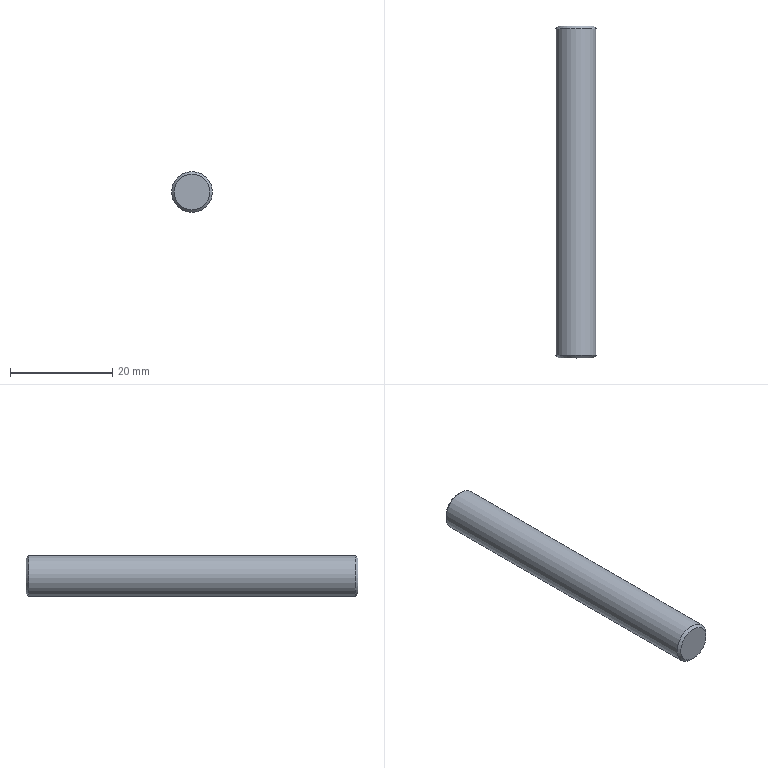Part | STEP file | 车灯-后视镜_id66_x_t | 1 solid | 5 faces | box 8 x 65 x 8 mm | volume 3261 mm3 | plane 2 | cone 2 | cylinder 1 | commonest cylinder face diameters 8 x1
STEP:
#1=CARTESIAN_POINT('',(-80.5,-260.,-279.));
#2=VERTEX_POINT('',#1);
#3=CARTESIAN_POINT('',(-80.5,-260.,-275.5));
#4=DIRECTION('',(0.,1.,0.));
#5=DIRECTION('',(0.,0.,-1.));
#6=AXIS2_PLACEMENT_3D('',#3,#4,#5);
#7=CIRCLE('',#6,3.5);
#8=EDGE_CURVE('',#2,#2,#7,.T.);
#9=ORIENTED_EDGE('',*,*,#8,.T.);
#10=EDGE_LOOP('',(#9));
#11=FACE_OUTER_BOUND('',#10,.T.);
#12=CARTESIAN_POINT('',(-80.5,-260.,-275.5));
#13=DIRECTION('',(0.,1.,0.));
#14=DIRECTION('',(0.,0.,1.));
#15=AXIS2_PLACEMENT_3D('',#12,#13,#14);
#16=PLANE('',#15);
#17=ADVANCED_FACE('',(#11),#16,.T.);
#18=CARTESIAN_POINT('',(-80.5,-325.,-272.));
#19=VERTEX_POINT('',#18);
#20=CARTESIAN_POINT('',(-80.5,-325.,-275.5));
#21=DIRECTION('',(0.,-1.,0.));
#22=DIRECTION('',(0.,0.,1.));
#23=AXIS2_PLACEMENT_3D('',#20,#21,#22);
#24=CIRCLE('',#23,3.5);
#25=EDGE_CURVE('',#19,#19,#24,.T.);
#26=ORIENTED_EDGE('',*,*,#25,.T.);
#27=EDGE_LOOP('',(#26));
#28=FACE_OUTER_BOUND('',#27,.T.);
#29=CARTESIAN_POINT('',(-80.5,-325.,-275.5));
#30=DIRECTION('',(0.,-1.,0.));
#31=DIRECTION('',(0.,0.,-1.));
#32=AXIS2_PLACEMENT_3D('',#29,#30,#31);
#33=PLANE('',#32);
#34=ADVANCED_FACE('',(#28),#33,.T.);
#35=CARTESIAN_POINT('',(-80.5,-324.5,-271.5));
#36=VERTEX_POINT('',#35);
#37=CARTESIAN_POINT('',(-80.5,-324.5,-275.5));
#38=DIRECTION('',(0.,1.,0.));
#39=DIRECTION('',(0.,0.,1.));
#40=AXIS2_PLACEMENT_3D('',#37,#38,#39);
#41=CIRCLE('',#40,4.);
#42=EDGE_CURVE('',#36,#36,#41,.T.);
#43=ORIENTED_EDGE('',*,*,#42,.T.);
#44=EDGE_LOOP('',(#43));
#45=FACE_BOUND('',#44,.T.);
#46=CARTESIAN_POINT('',(-80.5,-260.5,-279.5));
#47=VERTEX_POINT('',#46);
#48=CARTESIAN_POINT('',(-80.5,-260.5,-275.5));
#49=DIRECTION('',(0.,-1.,0.));
#50=DIRECTION('',(0.,0.,-1.));
#51=AXIS2_PLACEMENT_3D('',#48,#49,#50);
#52=CIRCLE('',#51,4.);
#53=EDGE_CURVE('',#47,#47,#52,.T.);
#54=ORIENTED_EDGE('',*,*,#53,.T.);
#55=EDGE_LOOP('',(#54));
#56=FACE_BOUND('',#55,.T.);
#57=CARTESIAN_POINT('',(-80.5,-325.,-275.5));
#58=DIRECTION('',(0.,1.,0.));
#59=DIRECTION('',(0.,0.,1.));
#60=AXIS2_PLACEMENT_3D('',#57,#58,#59);
#61=CYLINDRICAL_SURFACE('',#60,4.);
#62=ADVANCED_FACE('',(#45,#56),#61,.T.);
#63=ORIENTED_EDGE('',*,*,#25,.F.);
#64=EDGE_LOOP('',(#63));
#65=FACE_BOUND('',#64,.T.);
#66=ORIENTED_EDGE('',*,*,#42,.F.);
#67=EDGE_LOOP('',(#66));
#68=FACE_BOUND('',#67,.T.);
#69=CARTESIAN_POINT('',(-80.5,-324.5,-275.5));
#70=DIRECTION('',(0.,1.,0.));
#71=DIRECTION('',(0.,0.,-1.));
#72=AXIS2_PLACEMENT_3D('',#69,#70,#71);
#73=CONICAL_SURFACE('',#72,4.,45.);
#74=ADVANCED_FACE('',(#65,#68),#73,.T.);
#75=ORIENTED_EDGE('',*,*,#8,.F.);
#76=EDGE_LOOP('',(#75));
#77=FACE_BOUND('',#76,.T.);
#78=ORIENTED_EDGE('',*,*,#53,.F.);
#79=EDGE_LOOP('',(#78));
#80=FACE_BOUND('',#79,.T.);
#81=CARTESIAN_POINT('',(-80.5,-260.5,-275.5));
#82=DIRECTION('',(0.,-1.,0.));
#83=DIRECTION('',(0.,0.,1.));
#84=AXIS2_PLACEMENT_3D('',#81,#82,#83);
#85=CONICAL_SURFACE('',#84,4.,45.);
#86=ADVANCED_FACE('',(#77,#80),#85,.T.);
#87=CLOSED_SHELL('',(#17,#34,#62,#74,#86));
#88=MANIFOLD_SOLID_BREP('',#87);
#89=(LENGTH_UNIT()NAMED_UNIT(*)SI_UNIT(.MILLI.,.METRE.));
#90=UNCERTAINTY_MEASURE_WITH_UNIT(LENGTH_MEASURE(0.00002),#89,'','');
#91=(NAMED_UNIT(*)PLANE_ANGLE_UNIT()SI_UNIT($,.RADIAN.));
#92=PLANE_ANGLE_MEASURE_WITH_UNIT(PLANE_ANGLE_MEASURE(0.01745),#91);
#93=DIMENSIONAL_EXPONENTS(0.,0.,0.,0.,0.,0.,0.);
#94=(CONVERSION_BASED_UNIT('DEGREE',#92)NAMED_UNIT(#93)PLANE_ANGLE_UNIT());
#95=(NAMED_UNIT(*)SI_UNIT($,.STERADIAN.)SOLID_ANGLE_UNIT());
#96=(GEOMETRIC_REPRESENTATION_CONTEXT(3)GLOBAL_UNCERTAINTY_ASSIGNED_CONTEXT((#90))GLOBAL_UNIT_ASSIGNED_CONTEXT((#89,#94,#95))REPRESENTATION_CONTEXT('',''));
#97=ADVANCED_BREP_SHAPE_REPRESENTATION('',(#88),#96);